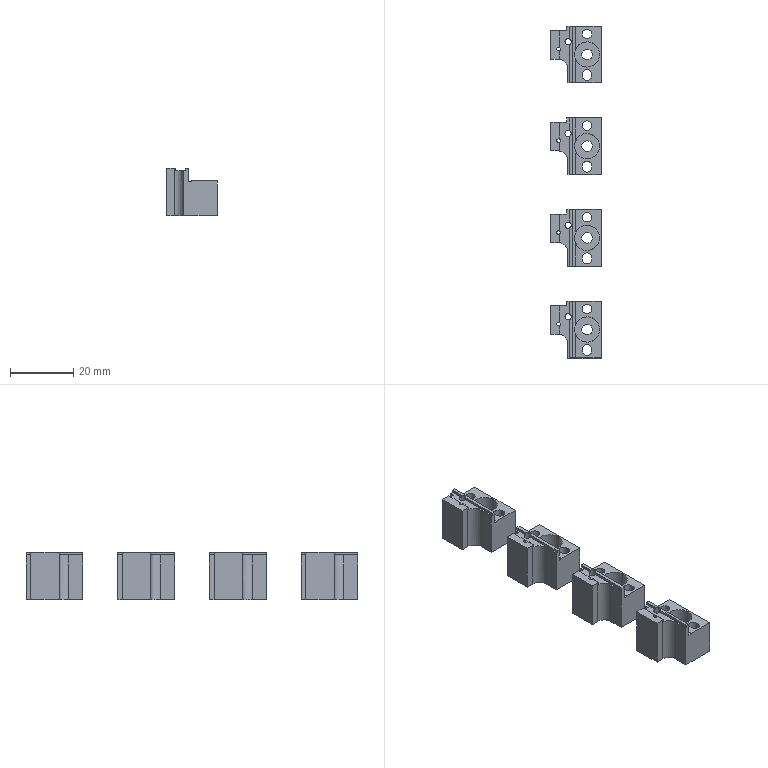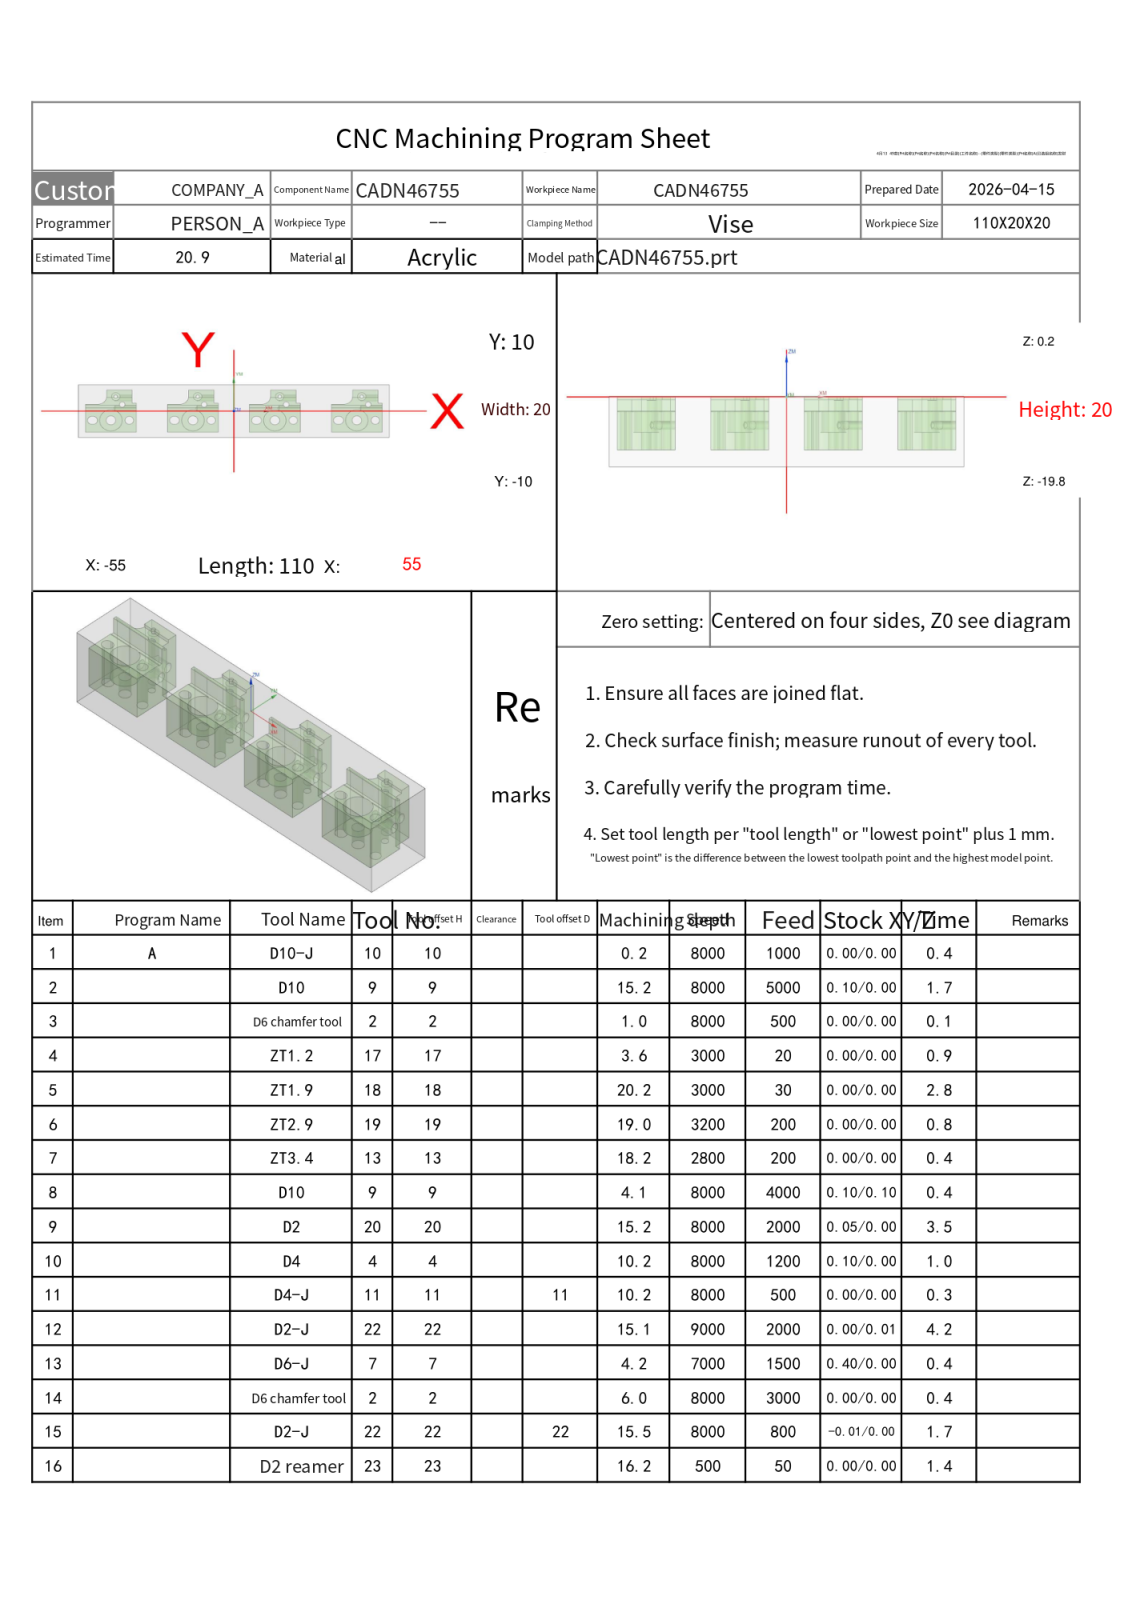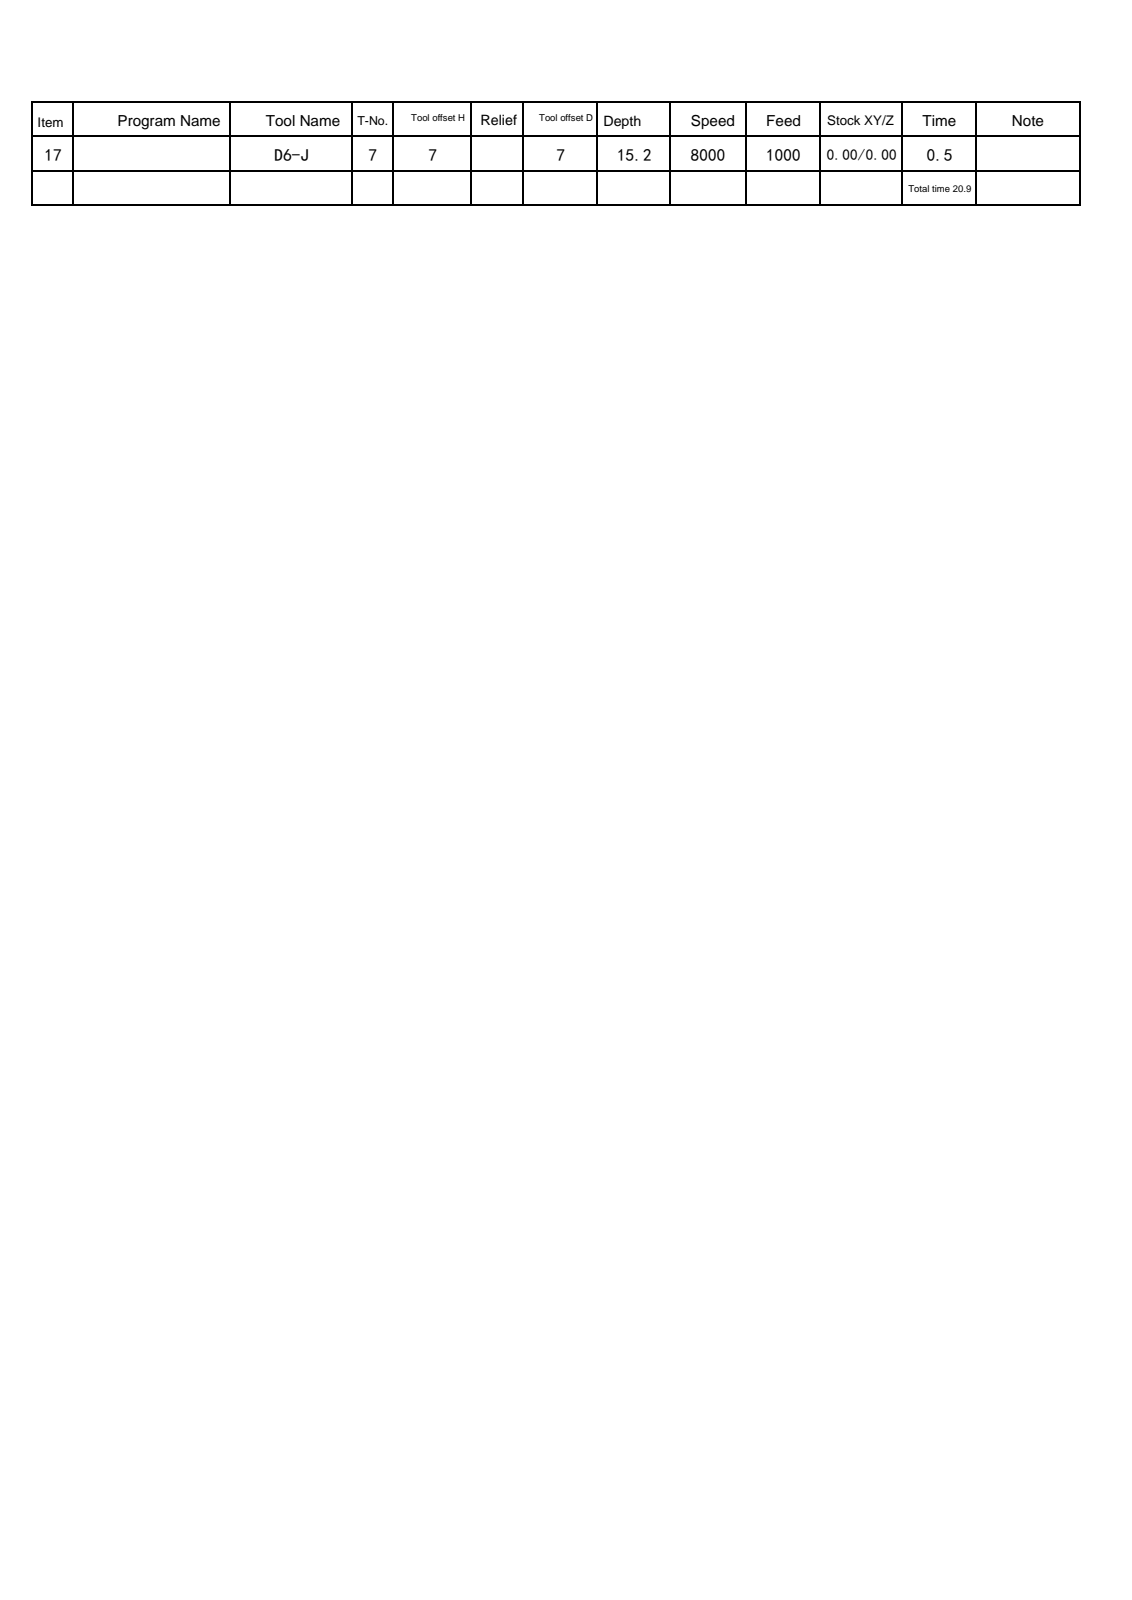NC program | NX | posted by the shop | part box 16 x 105 x 15 mm
Lines 5479 to 6592 of 25120:
N12 T22 M06
(D2-J  D=2. R=0. H=22 ce=0.00 di=0.01)
G00 G90 G54 X-46.858 Y4.697 M03 S9000
G43 H22 Z20.
M08
Z.601
G01 X-46.848 Z.486 F1600.
X-46.82 Y4.7 Z.384
X-46.778 Y4.706 Z.292
X-46.722 Y4.716 Z.211
X-46.657 Y4.731 Z.139
X-46.584 Y4.752 Z.077
X-46.506 Y4.779 Z.024
X-46.426 Y4.814 Z-.021
X-46.347 Y4.857 Z-.058
X-46.27 Y4.909 Z-.088
X-46.198 Y4.971 Z-.112
X-46.134 Y5.045 Z-.129
X-46.081 Y5.13 Z-.141
X-46.041 Y5.228 Z-.147
X-46.017 Y5.34 Z-.15
G03 X-46. Y5.6 I-1.983 J.26 F2000.
G01 Y7.3
X-46.007 Y7.322
X-46.026 Y7.315 Z-.153
X-46.054 Y7.283 Z-.157
X-46.089 Y7.228 Z-.162
X-46.128 Y7.154 Z-.168
X-46.167 Y7.064 Z-.174
X-46.205 Y6.96 Z-.182
X-46.239 Y6.847 Z-.19
X-46.286 Y6.601 Z-.207
X-46.304 Y6.34 Z-.224
X-46.293 Y6.077 Z-.242
X-46.254 Y5.825 Z-.259
X-46.223 Y5.707 Z-.267
X-46.188 Y5.599 Z-.274
X-46.15 Y5.503 Z-.281
X-46.113 Y5.424 Z-.287
X-46.078 Y5.365 Z-.292
X-46.049 Y5.329 Z-.296
X-46.028 Y5.319 Z-.298
X-46.017 Y5.34 Z-.299
G03 X-46. Y5.6 I-1.983 J.26
G01 Y7.3
X-46.007 Y7.322 Z-.3
X-46.026 Y7.315 Z-.302
X-46.054 Y7.283 Z-.306
X-46.089 Y7.228 Z-.311
X-46.128 Y7.154 Z-.317
X-46.167 Y7.064 Z-.324
X-46.205 Y6.96 Z-.331
X-46.239 Y6.847 Z-.339
X-46.286 Y6.601 Z-.356
X-46.304 Y6.34 Z-.374
X-46.293 Y6.077 Z-.391
X-46.254 Y5.825 Z-.408
X-46.223 Y5.707 Z-.416
X-46.188 Y5.599 Z-.424
X-46.15 Y5.503 Z-.43
X-46.113 Y5.424 Z-.436
X-46.078 Y5.365 Z-.441
X-46.049 Y5.329 Z-.445
X-46.028 Y5.319 Z-.448
X-46.017 Y5.34 Z-.449
G03 X-46. Y5.6 I-1.983 J.26
G01 Y7.3
X-46.007 Y7.322
X-46.026 Y7.315 Z-.452
X-46.054 Y7.283 Z-.456
X-46.089 Y7.228 Z-.461
X-46.128 Y7.154 Z-.467
X-46.167 Y7.064 Z-.473
X-46.205 Y6.96 Z-.481
X-46.239 Y6.847 Z-.489
X-46.286 Y6.601 Z-.506
X-46.304 Y6.34 Z-.523
X-46.293 Y6.077 Z-.541
X-46.254 Y5.825 Z-.558
X-46.223 Y5.707 Z-.566
X-46.188 Y5.599 Z-.573
X-46.15 Y5.503 Z-.58
X-46.113 Y5.424 Z-.586
X-46.078 Y5.365 Z-.591
X-46.049 Y5.329 Z-.595
X-46.028 Y5.319 Z-.597
X-46.017 Y5.34 Z-.598
G03 X-46. Y5.6 I-1.983 J.26
G01 Y7.3
X-46.007 Y7.322 Z-.599
X-46.026 Y7.315 Z-.601
X-46.054 Y7.283 Z-.605
X-46.089 Y7.228 Z-.61
X-46.128 Y7.154 Z-.616
X-46.167 Y7.064 Z-.623
X-46.205 Y6.96 Z-.63
X-46.239 Y6.847 Z-.638
X-46.286 Y6.601 Z-.655
X-46.304 Y6.34 Z-.673
X-46.293 Y6.077 Z-.69
X-46.254 Y5.825 Z-.707
X-46.223 Y5.707 Z-.715
X-46.188 Y5.599 Z-.723
X-46.15 Y5.503 Z-.729
X-46.113 Y5.424 Z-.735
X-46.078 Y5.365 Z-.74
X-46.049 Y5.329 Z-.744
X-46.028 Y5.319 Z-.747
X-46.017 Y5.34 Z-.748
G03 X-46. Y5.6 I-1.983 J.26
G01 Y7.3
X-46.016 Y7.315
X-46.061 Y7.307 Z-.749
X-46.132 Y7.278 Z-.751
X-46.228 Y7.23 Z-.754
X-46.483 Y7.077 Z-.762
X-46.829 Y6.848 Z-.773
X-47.215 Y6.572 Z-.785
X-47.805 Y6.108 Z-.805
X-48.29 Y5.688 Z-.822
X-48.757 Y5.248 Z-.84
X-49.231 Y4.758 Z-.858
X-49.573 Y4.37 Z-.872
X-49.839 Y4.044 Z-.883
X-50.012 Y3.809 Z-.89
X-50.068 Y3.722 Z-.893
X-50.102 Y3.656 Z-.895
X-50.113 Y3.614 Z-.897
X-50.1 Y3.6
X-48.
G03 X-46. Y5.6 I0.0 J2.
G01 Y7.7
X-46.016 Y7.713
X-46.061 Y7.702 Z-.899
X-46.132 Y7.668 Z-.901
X-46.227 Y7.612 Z-.904
X-46.545 Y7.393 Z-.913
X-46.84 Y7.17 Z-.922
X-47.213 Y6.871 Z-.934
X-47.803 Y6.354 Z-.954
X-48.289 Y5.887 Z-.972
X-48.755 Y5.402 Z-.989
X-49.272 Y4.812 Z-1.009
X-49.571 Y4.439 Z-1.021
X-49.794 Y4.144 Z-1.03
X-50.012 Y3.827 Z-1.04
X-50.068 Y3.732 Z-1.043
X-50.102 Y3.661 Z-1.045
X-50.113 Y3.616 Z-1.046
X-50.1 Y3.6 Z-1.047
X-48.
G03 X-46. Y5.6 I0.0 J2.
G01 Y7.7
X-46.016 Y7.713
X-46.061 Y7.702 Z-1.048
X-46.132 Y7.668 Z-1.05
X-46.227 Y7.612 Z-1.053
X-46.545 Y7.393 Z-1.063
X-46.84 Y7.17 Z-1.072
X-47.213 Y6.871 Z-1.084
X-47.803 Y6.354 Z-1.104
X-48.289 Y5.887 Z-1.121
X-48.755 Y5.402 Z-1.139
X-49.272 Y4.812 Z-1.159
X-49.571 Y4.439 Z-1.171
X-49.794 Y4.144 Z-1.18
X-50.012 Y3.827 Z-1.189
X-50.068 Y3.732 Z-1.192
X-50.102 Y3.661 Z-1.194
X-50.113 Y3.616 Z-1.196
X-50.1 Y3.6
X-48.
G03 X-46. Y5.6 I0.0 J2.
G01 Y7.7
X-46.016 Y7.713
X-46.061 Y7.702 Z-1.198
X-46.132 Y7.668 Z-1.2
X-46.227 Y7.612 Z-1.203
X-46.545 Y7.393 Z-1.212
X-46.84 Y7.17 Z-1.221
X-47.213 Y6.871 Z-1.233
X-47.803 Y6.354 Z-1.253
X-48.289 Y5.887 Z-1.271
X-48.755 Y5.402 Z-1.288
X-49.272 Y4.812 Z-1.308
X-49.571 Y4.439 Z-1.32
X-49.794 Y4.144 Z-1.329
X-50.012 Y3.827 Z-1.339
X-50.068 Y3.732 Z-1.342
X-50.102 Y3.661 Z-1.344
X-50.113 Y3.616 Z-1.345
X-50.1 Y3.6 Z-1.346
X-48.
G03 X-46. Y5.6 I0.0 J2.
G01 Y7.7
X-46.016 Y7.713
X-46.061 Y7.702 Z-1.347
X-46.132 Y7.668 Z-1.349
X-46.227 Y7.612 Z-1.352
X-46.545 Y7.393 Z-1.362
X-46.84 Y7.17 Z-1.371
X-47.213 Y6.871 Z-1.383
X-47.803 Y6.354 Z-1.403
X-48.289 Y5.887 Z-1.42
X-48.755 Y5.402 Z-1.438
X-49.272 Y4.812 Z-1.458
X-49.571 Y4.439 Z-1.47
X-49.794 Y4.144 Z-1.479
X-50.012 Y3.827 Z-1.488
X-50.068 Y3.732 Z-1.491
X-50.102 Y3.661 Z-1.493
X-50.113 Y3.616 Z-1.495
X-50.1 Y3.6
X-48.
G03 X-46. Y5.6 I0.0 J2.
G01 Y7.7
X-46.016 Y7.713
X-46.061 Y7.702 Z-1.497
X-46.132 Y7.668 Z-1.499
X-46.227 Y7.612 Z-1.502
X-46.545 Y7.393 Z-1.511
X-46.84 Y7.17 Z-1.52
X-47.213 Y6.871 Z-1.532
X-47.803 Y6.354 Z-1.552
X-48.289 Y5.887 Z-1.57
X-48.755 Y5.402 Z-1.587
X-49.272 Y4.812 Z-1.607
X-49.571 Y4.439 Z-1.619
X-49.794 Y4.144 Z-1.628
X-50.012 Y3.827 Z-1.638
X-50.068 Y3.732 Z-1.641
X-50.102 Y3.661 Z-1.643
X-50.113 Y3.616 Z-1.644
X-50.1 Y3.6 Z-1.645
X-48.
G03 X-46. Y5.6 I0.0 J2.
G01 Y7.7
X-46.016 Y7.713
X-46.061 Y7.702 Z-1.646
X-46.132 Y7.668 Z-1.648
X-46.227 Y7.612 Z-1.651
X-46.545 Y7.393 Z-1.661
X-46.84 Y7.17 Z-1.67
X-47.213 Y6.871 Z-1.682
X-47.803 Y6.354 Z-1.702
X-48.289 Y5.887 Z-1.719
X-48.755 Y5.402 Z-1.737
X-49.272 Y4.812 Z-1.757
X-49.571 Y4.439 Z-1.769
X-49.794 Y4.144 Z-1.778
X-50.012 Y3.827 Z-1.787
X-50.068 Y3.732 Z-1.79
X-50.102 Y3.661 Z-1.792
X-50.113 Y3.616 Z-1.794
X-50.1 Y3.6
X-48.
G03 X-46. Y5.6 I0.0 J2.
G01 Y7.7
X-46.016 Y7.713
X-46.061 Y7.702 Z-1.796
X-46.132 Y7.668 Z-1.798
X-46.227 Y7.612 Z-1.801
X-46.545 Y7.393 Z-1.81
X-46.84 Y7.17 Z-1.819
X-47.213 Y6.871 Z-1.831
X-47.803 Y6.354 Z-1.851
X-48.289 Y5.887 Z-1.869
X-48.755 Y5.402 Z-1.886
X-49.272 Y4.812 Z-1.906
X-49.571 Y4.439 Z-1.918
X-49.794 Y4.144 Z-1.927
X-50.012 Y3.827 Z-1.937
X-50.068 Y3.732 Z-1.94
X-50.102 Y3.661 Z-1.942
X-50.113 Y3.616 Z-1.943
X-50.1 Y3.6 Z-1.944
X-48.
G03 X-46. Y5.6 I0.0 J2.
G01 Y7.7
X-46.016 Y7.713
X-46.061 Y7.702 Z-1.945
X-46.132 Y7.668 Z-1.947
X-46.227 Y7.612 Z-1.95
X-46.545 Y7.393 Z-1.96
X-46.84 Y7.17 Z-1.969
X-47.213 Y6.871 Z-1.981
X-47.803 Y6.354 Z-2.001
X-48.289 Y5.887 Z-2.018
X-48.755 Y5.402 Z-2.036
X-49.272 Y4.812 Z-2.056
X-49.571 Y4.439 Z-2.068
X-49.794 Y4.144 Z-2.077
X-50.012 Y3.827 Z-2.086
X-50.068 Y3.732 Z-2.089
X-50.102 Y3.661 Z-2.091
X-50.113 Y3.616 Z-2.093
X-50.1 Y3.6
X-48.
G03 X-46. Y5.6 I0.0 J2.
G01 Y7.7
X-46.016 Y7.713
X-46.061 Y7.702 Z-2.095
X-46.132 Y7.668 Z-2.097
X-46.227 Y7.612 Z-2.1
X-46.545 Y7.393 Z-2.109
X-46.84 Y7.17 Z-2.118
X-47.213 Y6.871 Z-2.13
X-47.803 Y6.354 Z-2.15
X-48.289 Y5.887 Z-2.168
X-48.755 Y5.402 Z-2.185
X-49.272 Y4.812 Z-2.205
X-49.571 Y4.439 Z-2.217
X-49.794 Y4.144 Z-2.226
X-50.012 Y3.827 Z-2.236
X-50.068 Y3.732 Z-2.239
X-50.102 Y3.661 Z-2.241
X-50.113 Y3.616 Z-2.242
X-50.1 Y3.6 Z-2.243
X-48.
G03 X-46. Y5.6 I0.0 J2.
G01 Y7.7
X-46.016 Y7.713
X-46.061 Y7.702 Z-2.244
X-46.132 Y7.668 Z-2.246
X-46.227 Y7.612 Z-2.249
X-46.545 Y7.393 Z-2.259
X-46.84 Y7.17 Z-2.268
X-47.213 Y6.871 Z-2.28
X-47.803 Y6.354 Z-2.3
X-48.289 Y5.887 Z-2.317
X-48.755 Y5.402 Z-2.335
X-49.272 Y4.812 Z-2.355
X-49.571 Y4.439 Z-2.367
X-49.794 Y4.144 Z-2.376
X-50.012 Y3.827 Z-2.385
X-50.068 Y3.732 Z-2.388
X-50.102 Y3.661 Z-2.39
X-50.113 Y3.616 Z-2.392
X-50.1 Y3.6
X-48.
G03 X-46. Y5.6 I0.0 J2.
G01 Y7.7
X-46.016 Y7.713
X-46.061 Y7.702 Z-2.394
X-46.132 Y7.668 Z-2.396
X-46.227 Y7.612 Z-2.399
X-46.545 Y7.393 Z-2.408
X-46.84 Y7.17 Z-2.417
X-47.213 Y6.871 Z-2.429
X-47.803 Y6.354 Z-2.449
X-48.289 Y5.887 Z-2.467
X-48.755 Y5.402 Z-2.484
X-49.272 Y4.812 Z-2.504
X-49.571 Y4.439 Z-2.516
X-49.794 Y4.144 Z-2.525
X-50.012 Y3.827 Z-2.535
X-50.068 Y3.732 Z-2.538
X-50.102 Y3.661 Z-2.54
X-50.113 Y3.616 Z-2.541
X-50.1 Y3.6 Z-2.542
X-48.
G03 X-46. Y5.6 I0.0 J2.
G01 Y7.7
X-46.016 Y7.713
X-46.061 Y7.702 Z-2.543
X-46.132 Y7.668 Z-2.545
X-46.227 Y7.612 Z-2.548
X-46.545 Y7.393 Z-2.558
X-46.84 Y7.17 Z-2.567
X-47.213 Y6.871 Z-2.579
X-47.803 Y6.354 Z-2.599
X-48.289 Y5.887 Z-2.616
X-48.755 Y5.402 Z-2.634
X-49.272 Y4.812 Z-2.654
X-49.571 Y4.439 Z-2.666
X-49.794 Y4.144 Z-2.675
X-50.012 Y3.827 Z-2.684
X-50.068 Y3.732 Z-2.687
X-50.102 Y3.661 Z-2.689
X-50.113 Y3.616 Z-2.691
X-50.1 Y3.6
X-48.
G03 X-46. Y5.6 I0.0 J2.
G01 Y7.7
X-46.016 Y7.713
X-46.061 Y7.702 Z-2.693
X-46.132 Y7.668 Z-2.695
X-46.227 Y7.612 Z-2.698
X-46.545 Y7.393 Z-2.707
X-46.84 Y7.17 Z-2.716
X-47.213 Y6.871 Z-2.728
X-47.803 Y6.354 Z-2.748
X-48.289 Y5.887 Z-2.766
X-48.755 Y5.402 Z-2.783
X-49.272 Y4.812 Z-2.803
X-49.571 Y4.439 Z-2.815
X-49.794 Y4.144 Z-2.824
X-50.012 Y3.827 Z-2.834
X-50.068 Y3.732 Z-2.837
X-50.102 Y3.661 Z-2.839
X-50.113 Y3.616 Z-2.84
X-50.1 Y3.6 Z-2.841
X-48.
G03 X-46. Y5.6 I0.0 J2.
G01 Y7.7
X-46.016 Y7.713
X-46.061 Y7.702 Z-2.842
X-46.132 Y7.668 Z-2.844
X-46.227 Y7.612 Z-2.847
X-46.545 Y7.393 Z-2.857
X-46.84 Y7.17 Z-2.866
X-47.213 Y6.871 Z-2.878
X-47.803 Y6.354 Z-2.898
X-48.289 Y5.887 Z-2.915
X-48.755 Y5.402 Z-2.933
X-49.272 Y4.812 Z-2.953
X-49.571 Y4.439 Z-2.965
X-49.794 Y4.144 Z-2.974
X-50.012 Y3.827 Z-2.983
X-50.068 Y3.732 Z-2.986
X-50.102 Y3.661 Z-2.988
X-50.113 Y3.616 Z-2.99
X-50.1 Y3.6
X-48.
G03 X-46. Y5.6 I0.0 J2.
G01 Y7.7
X-46.016 Y7.713
X-46.061 Y7.702 Z-2.992
X-46.132 Y7.668 Z-2.994
X-46.227 Y7.612 Z-2.997
X-46.545 Y7.393 Z-3.006
X-46.84 Y7.17 Z-3.015
X-47.213 Y6.871 Z-3.027
X-47.803 Y6.354 Z-3.047
X-48.289 Y5.887 Z-3.065
X-48.755 Y5.402 Z-3.082
X-49.272 Y4.812 Z-3.102
X-49.571 Y4.439 Z-3.114
X-49.794 Y4.144 Z-3.123
X-50.012 Y3.827 Z-3.133
X-50.068 Y3.732 Z-3.136
X-50.102 Y3.661 Z-3.138
X-50.113 Y3.616 Z-3.139
X-50.1 Y3.6 Z-3.14
X-48.
G03 X-46. Y5.6 I0.0 J2.
G01 Y7.7
X-46.016 Y7.713
X-46.061 Y7.702 Z-3.141
X-46.132 Y7.668 Z-3.143
X-46.227 Y7.612 Z-3.146
X-46.545 Y7.393 Z-3.156
X-46.84 Y7.17 Z-3.165
X-47.213 Y6.871 Z-3.177
X-47.803 Y6.354 Z-3.197
X-48.289 Y5.887 Z-3.214
X-48.755 Y5.402 Z-3.232
X-49.272 Y4.812 Z-3.252
X-49.571 Y4.439 Z-3.264
X-49.794 Y4.144 Z-3.273
X-50.012 Y3.827 Z-3.282
X-50.068 Y3.732 Z-3.285
X-50.102 Y3.661 Z-3.287
X-50.113 Y3.616 Z-3.289
X-50.1 Y3.6
X-48.
G03 X-46. Y5.6 I0.0 J2.
G01 Y7.7
X-46.016 Y7.713
X-46.061 Y7.702 Z-3.291
X-46.132 Y7.668 Z-3.293
X-46.227 Y7.612 Z-3.296
X-46.545 Y7.393 Z-3.305
X-46.84 Y7.17 Z-3.314
X-47.213 Y6.871 Z-3.326
X-47.803 Y6.354 Z-3.346
X-48.289 Y5.887 Z-3.364
X-48.755 Y5.402 Z-3.381
X-49.272 Y4.812 Z-3.401
X-49.571 Y4.439 Z-3.413
X-49.794 Y4.144 Z-3.422
X-50.012 Y3.827 Z-3.432
X-50.068 Y3.732 Z-3.435
X-50.102 Y3.661 Z-3.437
X-50.113 Y3.616 Z-3.438
X-50.1 Y3.6 Z-3.439
X-48.
G03 X-46. Y5.6 I0.0 J2.
G01 Y7.7
X-46.016 Y7.713
X-46.061 Y7.702 Z-3.44
X-46.132 Y7.668 Z-3.442
X-46.227 Y7.612 Z-3.445
X-46.545 Y7.393 Z-3.455
X-46.84 Y7.17 Z-3.464
X-47.213 Y6.871 Z-3.476
X-47.803 Y6.354 Z-3.496
X-48.289 Y5.887 Z-3.513
X-48.755 Y5.402 Z-3.531
X-49.272 Y4.812 Z-3.551
X-49.571 Y4.439 Z-3.563
X-49.794 Y4.144 Z-3.572
X-50.012 Y3.827 Z-3.581
X-50.068 Y3.732 Z-3.584
X-50.102 Y3.661 Z-3.586
X-50.113 Y3.616 Z-3.588
X-50.1 Y3.6
X-48.
G03 X-46. Y5.6 I0.0 J2.
G01 Y7.7
X-46.016 Y7.713
X-46.061 Y7.702 Z-3.59
X-46.132 Y7.668 Z-3.592
X-46.227 Y7.612 Z-3.595
X-46.545 Y7.393 Z-3.604
X-46.84 Y7.17 Z-3.613
X-47.213 Y6.871 Z-3.625
X-47.803 Y6.354 Z-3.645
X-48.289 Y5.887 Z-3.663
X-48.755 Y5.402 Z-3.68
X-49.272 Y4.812 Z-3.7
X-49.571 Y4.439 Z-3.712
X-49.794 Y4.144 Z-3.721
X-50.012 Y3.827 Z-3.731
X-50.068 Y3.732 Z-3.734
X-50.102 Y3.661 Z-3.736
X-50.113 Y3.616 Z-3.737
X-50.1 Y3.6 Z-3.738
X-48.
G03 X-46. Y5.6 I0.0 J2.
G01 Y7.7
X-46.016 Y7.713
X-46.061 Y7.702 Z-3.739
X-46.132 Y7.668 Z-3.741
X-46.227 Y7.612 Z-3.744
X-46.545 Y7.393 Z-3.754
X-46.84 Y7.17 Z-3.763
X-47.213 Y6.871 Z-3.775
X-47.803 Y6.354 Z-3.795
X-48.289 Y5.887 Z-3.812
X-48.755 Y5.402 Z-3.83
X-49.272 Y4.812 Z-3.85
X-49.571 Y4.439 Z-3.862
X-49.794 Y4.144 Z-3.871
X-50.012 Y3.827 Z-3.88
X-50.068 Y3.732 Z-3.883
X-50.102 Y3.661 Z-3.885
X-50.113 Y3.616 Z-3.887
X-50.1 Y3.6
X-48.
G03 X-46. Y5.6 I0.0 J2.
G01 Y7.7
X-46.016 Y7.713
X-46.061 Y7.702 Z-3.889
X-46.132 Y7.668 Z-3.891
X-46.227 Y7.612 Z-3.894
X-46.545 Y7.393 Z-3.903
X-46.84 Y7.17 Z-3.912
X-47.213 Y6.871 Z-3.924
X-47.803 Y6.354 Z-3.944
X-48.289 Y5.887 Z-3.962
X-48.755 Y5.402 Z-3.979
X-49.272 Y4.812 Z-3.999
X-49.571 Y4.439 Z-4.011
X-49.794 Y4.144 Z-4.02
X-50.012 Y3.827 Z-4.03
X-50.068 Y3.732 Z-4.033
X-50.102 Y3.661 Z-4.035
X-50.113 Y3.616 Z-4.036
X-50.1 Y3.6 Z-4.037
X-48.
G03 X-46. Y5.6 I0.0 J2.
G01 Y7.7
X-46.016 Y7.713
X-46.061 Y7.702 Z-4.038
X-46.132 Y7.668 Z-4.04
X-46.227 Y7.612 Z-4.043
X-46.545 Y7.393 Z-4.053
X-46.84 Y7.17 Z-4.062
X-47.213 Y6.871 Z-4.074
X-47.803 Y6.354 Z-4.094
X-48.289 Y5.887 Z-4.111
X-48.755 Y5.402 Z-4.129
X-49.272 Y4.812 Z-4.149
X-49.571 Y4.439 Z-4.161
X-49.794 Y4.144 Z-4.17
X-50.012 Y3.827 Z-4.179
X-50.068 Y3.732 Z-4.182
X-50.102 Y3.661 Z-4.184
X-50.113 Y3.616 Z-4.186
X-50.1 Y3.6
X-48.
G03 X-46. Y5.6 I0.0 J2.
G01 Y7.7
X-46.016 Y7.713
X-46.061 Y7.702 Z-4.188
X-46.132 Y7.668 Z-4.19
X-46.227 Y7.612 Z-4.193
X-46.545 Y7.393 Z-4.202
X-46.84 Y7.17 Z-4.211
X-47.213 Y6.871 Z-4.223
X-47.803 Y6.354 Z-4.243
X-48.289 Y5.887 Z-4.261
X-48.755 Y5.402 Z-4.278
X-49.272 Y4.812 Z-4.298
X-49.571 Y4.439 Z-4.31
X-49.794 Y4.144 Z-4.319
X-50.012 Y3.827 Z-4.329
X-50.068 Y3.732 Z-4.332
X-50.102 Y3.661 Z-4.334
X-50.113 Y3.616 Z-4.335
X-50.1 Y3.6 Z-4.336
X-48.
G03 X-46. Y5.6 I0.0 J2.
G01 Y7.7
X-46.016 Y7.713
X-46.061 Y7.702 Z-4.337
X-46.132 Y7.668 Z-4.339
X-46.227 Y7.612 Z-4.342
X-46.545 Y7.393 Z-4.352
X-46.84 Y7.17 Z-4.361
X-47.213 Y6.871 Z-4.373
X-47.803 Y6.354 Z-4.393
X-48.289 Y5.887 Z-4.41
X-48.755 Y5.402 Z-4.428
X-49.272 Y4.812 Z-4.448
X-49.571 Y4.439 Z-4.46
X-49.794 Y4.144 Z-4.469
X-50.012 Y3.827 Z-4.478
X-50.068 Y3.732 Z-4.481
X-50.102 Y3.661 Z-4.483
X-50.113 Y3.616 Z-4.485
X-50.1 Y3.6
X-48.
G03 X-46. Y5.6 I0.0 J2.
G01 Y7.7
X-46.016 Y7.713
X-46.061 Y7.702 Z-4.487
X-46.132 Y7.668 Z-4.489
X-46.227 Y7.612 Z-4.492
X-46.545 Y7.393 Z-4.501
X-46.84 Y7.17 Z-4.51
X-47.213 Y6.871 Z-4.522
X-47.803 Y6.354 Z-4.542
X-48.289 Y5.887 Z-4.56
X-48.755 Y5.402 Z-4.577
X-49.272 Y4.812 Z-4.597
X-49.571 Y4.439 Z-4.609
X-49.794 Y4.144 Z-4.618
X-50.012 Y3.827 Z-4.628
X-50.068 Y3.732 Z-4.631
X-50.102 Y3.661 Z-4.633
X-50.113 Y3.616 Z-4.634
X-50.1 Y3.6 Z-4.635
X-48.
G03 X-46. Y5.6 I0.0 J2.
G01 Y7.7
X-46.016 Y7.713
X-46.061 Y7.702 Z-4.636
X-46.132 Y7.668 Z-4.638
X-46.227 Y7.612 Z-4.641
X-46.545 Y7.393 Z-4.651
X-46.84 Y7.17 Z-4.66
X-47.213 Y6.871 Z-4.672
X-47.803 Y6.354 Z-4.692
X-48.289 Y5.887 Z-4.709
X-48.755 Y5.402 Z-4.727
X-49.272 Y4.812 Z-4.747
X-49.571 Y4.439 Z-4.759
X-49.794 Y4.144 Z-4.768
X-50.012 Y3.827 Z-4.777
X-50.068 Y3.732 Z-4.78
X-50.102 Y3.661 Z-4.782
X-50.113 Y3.616 Z-4.784
X-50.1 Y3.6
X-48.
G03 X-46. Y5.6 I0.0 J2.
G01 Y7.7
X-46.016 Y7.713
X-46.061 Y7.702 Z-4.786
X-46.132 Y7.668 Z-4.788
X-46.227 Y7.612 Z-4.791
X-46.545 Y7.393 Z-4.8
X-46.84 Y7.17 Z-4.809
X-47.213 Y6.871 Z-4.821
X-47.803 Y6.354 Z-4.841
X-48.289 Y5.887 Z-4.859
X-48.755 Y5.402 Z-4.876
X-49.272 Y4.812 Z-4.896
X-49.571 Y4.439 Z-4.908
X-49.794 Y4.144 Z-4.917
X-50.012 Y3.827 Z-4.927
X-50.068 Y3.732 Z-4.93
X-50.102 Y3.661 Z-4.932
X-50.113 Y3.616 Z-4.933
X-50.1 Y3.6 Z-4.934
X-48.
G03 X-46. Y5.6 I0.0 J2.
G01 Y7.7
X-46.016 Y7.713
X-46.061 Y7.702 Z-4.935
X-46.132 Y7.668 Z-4.937
X-46.227 Y7.612 Z-4.94
X-46.545 Y7.393 Z-4.95
X-46.84 Y7.17 Z-4.959
X-47.213 Y6.871 Z-4.971
X-47.803 Y6.354 Z-4.991
X-48.289 Y5.887 Z-5.008
X-48.755 Y5.402 Z-5.026
X-49.272 Y4.812 Z-5.046
X-49.571 Y4.439 Z-5.058
X-49.794 Y4.144 Z-5.067
X-50.012 Y3.827 Z-5.076
X-50.068 Y3.732 Z-5.079
X-50.102 Y3.661 Z-5.081
X-50.113 Y3.616 Z-5.083
X-50.1 Y3.6
X-48.
G03 X-46. Y5.6 I0.0 J2.
G01 Y7.7
X-46.016 Y7.713
X-46.061 Y7.702 Z-5.085
X-46.132 Y7.668 Z-5.087
X-46.227 Y7.612 Z-5.09
X-46.545 Y7.393 Z-5.099
X-46.84 Y7.17 Z-5.108
X-47.213 Y6.871 Z-5.12
X-47.803 Y6.354 Z-5.14
X-48.289 Y5.887 Z-5.158
X-48.755 Y5.402 Z-5.175
X-49.272 Y4.812 Z-5.195
X-49.571 Y4.439 Z-5.207
X-49.794 Y4.144 Z-5.216
X-50.012 Y3.827 Z-5.226
X-50.068 Y3.732 Z-5.229
X-50.102 Y3.661 Z-5.231
X-50.113 Y3.616 Z-5.232
X-50.1 Y3.6 Z-5.233
X-48.
G03 X-46. Y5.6 I0.0 J2.
G01 Y7.7
X-46.016 Y7.713
X-46.061 Y7.702 Z-5.234
X-46.132 Y7.668 Z-5.236
X-46.227 Y7.612 Z-5.239
X-46.545 Y7.393 Z-5.249
X-46.84 Y7.17 Z-5.258
X-47.213 Y6.871 Z-5.27
X-47.803 Y6.354 Z-5.29
X-48.289 Y5.887 Z-5.307
X-48.755 Y5.402 Z-5.325
X-49.272 Y4.812 Z-5.345
X-49.571 Y4.439 Z-5.357
X-49.794 Y4.144 Z-5.366
X-50.012 Y3.827 Z-5.375
X-50.068 Y3.732 Z-5.378
X-50.102 Y3.661 Z-5.38
X-50.113 Y3.616 Z-5.382
X-50.1 Y3.6
X-48.
G03 X-46. Y5.6 I0.0 J2.
G01 Y7.7
X-46.016 Y7.713
X-46.061 Y7.702 Z-5.384
X-46.132 Y7.668 Z-5.386
X-46.227 Y7.612 Z-5.389
X-46.545 Y7.393 Z-5.398
X-46.84 Y7.17 Z-5.407
X-47.213 Y6.871 Z-5.419
X-47.803 Y6.354 Z-5.439
X-48.289 Y5.887 Z-5.457
X-48.755 Y5.402 Z-5.474
X-49.272 Y4.812 Z-5.494
X-49.571 Y4.439 Z-5.506
X-49.794 Y4.144 Z-5.515
X-50.012 Y3.827 Z-5.525
X-50.068 Y3.732 Z-5.528
X-50.102 Y3.661 Z-5.53
X-50.113 Y3.616 Z-5.531
X-50.1 Y3.6 Z-5.532
X-48.
G03 X-46. Y5.6 I0.0 J2.
G01 Y7.7
X-46.016 Y7.713
X-46.061 Y7.702 Z-5.533
X-46.132 Y7.668 Z-5.535
X-46.227 Y7.612 Z-5.538
X-46.545 Y7.393 Z-5.548
X-46.84 Y7.17 Z-5.557
X-47.213 Y6.871 Z-5.569
X-47.803 Y6.354 Z-5.589
X-48.289 Y5.887 Z-5.606
X-48.755 Y5.402 Z-5.624
X-49.272 Y4.812 Z-5.644
X-49.571 Y4.439 Z-5.656
X-49.794 Y4.144 Z-5.665
X-50.012 Y3.827 Z-5.674
X-50.068 Y3.732 Z-5.677
X-50.102 Y3.661 Z-5.679
X-50.113 Y3.616 Z-5.681
X-50.1 Y3.6
X-48.
G03 X-46. Y5.6 I0.0 J2.
G01 Y7.7
X-46.016 Y7.713
X-46.061 Y7.702 Z-5.683
X-46.132 Y7.668 Z-5.685
X-46.227 Y7.612 Z-5.688
X-46.545 Y7.393 Z-5.697
X-46.84 Y7.17 Z-5.706
X-47.213 Y6.871 Z-5.718
X-47.803 Y6.354 Z-5.738
X-48.289 Y5.887 Z-5.756
X-48.755 Y5.402 Z-5.773
X-49.272 Y4.812 Z-5.793
X-49.571 Y4.439 Z-5.805
X-49.794 Y4.144 Z-5.814
X-50.012 Y3.827 Z-5.824
X-50.068 Y3.732 Z-5.827
X-50.102 Y3.661 Z-5.829
X-50.113 Y3.616 Z-5.83
X-50.1 Y3.6 Z-5.831
X-48.
G03 X-46. Y5.6 I0.0 J2.
G01 Y7.7
X-46.016 Y7.713
X-46.061 Y7.702 Z-5.832
X-46.132 Y7.668 Z-5.834
X-46.227 Y7.612 Z-5.837
X-46.545 Y7.393 Z-5.847
X-46.84 Y7.17 Z-5.856
X-47.213 Y6.871 Z-5.868
X-47.803 Y6.354 Z-5.888
X-48.289 Y5.887 Z-5.905
X-48.755 Y5.402 Z-5.923
X-49.272 Y4.812 Z-5.943
X-49.571 Y4.439 Z-5.955
X-49.794 Y4.144 Z-5.964
X-50.012 Y3.827 Z-5.973
X-50.068 Y3.732 Z-5.976
X-50.102 Y3.661 Z-5.978
X-50.113 Y3.616 Z-5.98
X-50.1 Y3.6
X-48.
G03 X-46. Y5.6 I0.0 J2.
G01 Y7.7
X-46.016 Y7.713
X-46.061 Y7.702 Z-5.982
X-46.132 Y7.668 Z-5.984
X-46.227 Y7.612 Z-5.987
X-46.545 Y7.393 Z-5.996
X-46.84 Y7.17 Z-6.005
X-47.213 Y6.871 Z-6.017
X-47.803 Y6.354 Z-6.037
X-48.289 Y5.887 Z-6.055
X-48.755 Y5.402 Z-6.072
X-49.272 Y4.812 Z-6.092
X-49.571 Y4.439 Z-6.104
X-49.794 Y4.144 Z-6.113
X-50.012 Y3.827 Z-6.123
X-50.068 Y3.732 Z-6.126
X-50.102 Y3.661 Z-6.128
X-50.113 Y3.616 Z-6.129
X-50.1 Y3.6 Z-6.13
X-48.
G03 X-46. Y5.6 I0.0 J2.
G01 Y7.7
X-46.016 Y7.713
X-46.061 Y7.702 Z-6.131
X-46.132 Y7.668 Z-6.133
X-46.227 Y7.612 Z-6.136
X-46.545 Y7.393 Z-6.146
X-46.84 Y7.17 Z-6.155
X-47.213 Y6.871 Z-6.167
X-47.803 Y6.354 Z-6.187
X-48.289 Y5.887 Z-6.204
X-48.755 Y5.402 Z-6.222
X-49.272 Y4.812 Z-6.242
X-49.571 Y4.439 Z-6.254
X-49.794 Y4.144 Z-6.263
X-50.012 Y3.827 Z-6.272
X-50.068 Y3.732 Z-6.275
X-50.102 Y3.661 Z-6.277
X-50.113 Y3.616 Z-6.279
X-50.1 Y3.6
X-48.
G03 X-46. Y5.6 I0.0 J2.
G01 Y7.7
X-46.016 Y7.713
X-46.061 Y7.702 Z-6.281
X-46.132 Y7.668 Z-6.283
X-46.227 Y7.612 Z-6.286
X-46.545 Y7.393 Z-6.295
X-46.84 Y7.17 Z-6.304
X-47.213 Y6.871 Z-6.316
X-47.803 Y6.354 Z-6.336
X-48.289 Y5.887 Z-6.354
X-48.755 Y5.402 Z-6.371
X-49.272 Y4.812 Z-6.391
X-49.571 Y4.439 Z-6.403
X-49.794 Y4.144 Z-6.412
X-50.012 Y3.827 Z-6.422
X-50.068 Y3.732 Z-6.425
X-50.102 Y3.661 Z-6.427
X-50.113 Y3.616 Z-6.428
X-50.1 Y3.6 Z-6.429
X-48.
G03 X-46. Y5.6 I0.0 J2.
G01 Y7.7
X-46.016 Y7.713
X-46.061 Y7.702 Z-6.43
X-46.132 Y7.668 Z-6.432
X-46.227 Y7.612 Z-6.435
X-46.545 Y7.393 Z-6.445
X-46.84 Y7.17 Z-6.454
X-47.213 Y6.871 Z-6.466
X-47.803 Y6.354 Z-6.486
X-48.289 Y5.887 Z-6.503
X-48.755 Y5.402 Z-6.521
X-49.272 Y4.812 Z-6.541
X-49.571 Y4.439 Z-6.553
X-49.794 Y4.144 Z-6.562
X-50.012 Y3.827 Z-6.571
X-50.068 Y3.732 Z-6.574
X-50.102 Y3.661 Z-6.576
X-50.113 Y3.616 Z-6.578
X-50.1 Y3.6
X-48.
G03 X-46. Y5.6 I0.0 J2.
G01 Y7.7
X-46.016 Y7.713
X-46.061 Y7.702 Z-6.58
X-46.132 Y7.668 Z-6.582
X-46.227 Y7.612 Z-6.585
X-46.545 Y7.393 Z-6.594
X-46.84 Y7.17 Z-6.603
X-47.213 Y6.871 Z-6.615
X-47.803 Y6.354 Z-6.635
X-48.289 Y5.887 Z-6.653
X-48.755 Y5.402 Z-6.67
X-49.272 Y4.812 Z-6.69
X-49.571 Y4.439 Z-6.702
X-49.794 Y4.144 Z-6.711
X-50.012 Y3.827 Z-6.721
X-50.068 Y3.732 Z-6.724
X-50.102 Y3.661 Z-6.726
X-50.113 Y3.616 Z-6.727
X-50.1 Y3.6 Z-6.728
X-48.
G03 X-46. Y5.6 I0.0 J2.
G01 Y7.7
X-46.016 Y7.713
X-46.061 Y7.702 Z-6.729
X-46.132 Y7.668 Z-6.731
X-46.227 Y7.612 Z-6.734
X-46.545 Y7.393 Z-6.744
X-46.84 Y7.17 Z-6.753
X-47.213 Y6.871 Z-6.765
X-47.803 Y6.354 Z-6.785
X-48.289 Y5.887 Z-6.802
X-48.755 Y5.402 Z-6.82
X-49.272 Y4.812 Z-6.84
X-49.571 Y4.439 Z-6.852
X-49.794 Y4.144 Z-6.861
X-50.012 Y3.827 Z-6.87
X-50.068 Y3.732 Z-6.873
X-50.102 Y3.661 Z-6.875
X-50.113 Y3.616 Z-6.877
X-50.1 Y3.6
X-48.
G03 X-46. Y5.6 I0.0 J2.
G01 Y7.7
X-46.016 Y7.713
X-46.061 Y7.702 Z-6.879
X-46.132 Y7.668 Z-6.881
X-46.227 Y7.612 Z-6.884
X-46.545 Y7.393 Z-6.893
X-46.84 Y7.17 Z-6.902
X-47.213 Y6.871 Z-6.914
X-47.803 Y6.354 Z-6.934
X-48.289 Y5.887 Z-6.952
X-48.755 Y5.402 Z-6.969
X-49.272 Y4.812 Z-6.989
X-49.571 Y4.439 Z-7.001
X-49.794 Y4.144 Z-7.01
X-50.012 Y3.827 Z-7.02
X-50.068 Y3.732 Z-7.023
X-50.102 Y3.661 Z-7.025
X-50.113 Y3.616 Z-7.026
X-50.1 Y3.6 Z-7.027
X-48.
G03 X-46. Y5.6 I0.0 J2.
G01 Y7.7
X-46.016 Y7.713
X-46.061 Y7.702 Z-7.028
X-46.132 Y7.668 Z-7.03
X-46.227 Y7.612 Z-7.033
X-46.545 Y7.393 Z-7.043
X-46.84 Y7.17 Z-7.052
X-47.213 Y6.871 Z-7.064
X-47.803 Y6.354 Z-7.084
X-48.289 Y5.887 Z-7.101
X-48.755 Y5.402 Z-7.119
X-49.272 Y4.812 Z-7.139
X-49.571 Y4.439 Z-7.151
X-49.794 Y4.144 Z-7.16
X-50.012 Y3.827 Z-7.169
X-50.068 Y3.732 Z-7.172
X-50.102 Y3.661 Z-7.174
X-50.113 Y3.616 Z-7.176
X-50.1 Y3.6
X-48.
G03 X-46. Y5.6 I0.0 J2.
G01 Y7.7
X-46.016 Y7.713
X-46.061 Y7.702 Z-7.178
X-46.132 Y7.668 Z-7.18
X-46.227 Y7.612 Z-7.183
X-46.545 Y7.393 Z-7.192
X-46.84 Y7.17 Z-7.201
X-47.213 Y6.871 Z-7.213
X-47.803 Y6.354 Z-7.233
X-48.289 Y5.887 Z-7.251
X-48.755 Y5.402 Z-7.268
X-49.272 Y4.812 Z-7.288
X-49.571 Y4.439 Z-7.3
X-49.794 Y4.144 Z-7.309
X-50.012 Y3.827 Z-7.319
X-50.068 Y3.732 Z-7.322
X-50.102 Y3.661 Z-7.324
X-50.113 Y3.616 Z-7.325
X-50.1 Y3.6 Z-7.326
X-48.
G03 X-46. Y5.6 I0.0 J2.
G01 Y7.7
X-46.016 Y7.713
X-46.061 Y7.702 Z-7.327
X-46.132 Y7.668 Z-7.329
X-46.227 Y7.612 Z-7.332
X-46.545 Y7.393 Z-7.342
X-46.84 Y7.17 Z-7.351
X-47.213 Y6.871 Z-7.363
X-47.803 Y6.354 Z-7.383
X-48.289 Y5.887 Z-7.4
X-48.755 Y5.402 Z-7.418
X-49.272 Y4.812 Z-7.438
X-49.571 Y4.439 Z-7.45
X-49.794 Y4.144 Z-7.459
X-50.012 Y3.827 Z-7.468
X-50.068 Y3.732 Z-7.471
X-50.102 Y3.661 Z-7.473
X-50.113 Y3.616 Z-7.475
X-50.1 Y3.6
X-48.
G03 X-46. Y5.6 I0.0 J2.
G01 Y7.7
X-46.016 Y7.713
X-46.061 Y7.702 Z-7.477
X-46.132 Y7.668 Z-7.479
X-46.227 Y7.612 Z-7.482
X-46.545 Y7.393 Z-7.491
X-46.84 Y7.17 Z-7.5
X-47.213 Y6.871 Z-7.512
X-47.803 Y6.354 Z-7.532
X-48.289 Y5.887 Z-7.55
X-48.755 Y5.402 Z-7.567
X-49.272 Y4.812 Z-7.587
X-49.571 Y4.439 Z-7.599
X-49.794 Y4.144 Z-7.608
X-50.012 Y3.827 Z-7.618
X-50.068 Y3.732 Z-7.621
X-50.102 Y3.661 Z-7.623
X-50.113 Y3.616 Z-7.624
X-50.1 Y3.6 Z-7.625
X-48.
G03 X-46. Y5.6 I0.0 J2.
G01 Y7.7
X-46.016 Y7.713
X-46.061 Y7.702 Z-7.626
X-46.132 Y7.668 Z-7.628
X-46.227 Y7.612 Z-7.631
X-46.545 Y7.393 Z-7.641
X-46.84 Y7.17 Z-7.65
X-47.213 Y6.871 Z-7.662
X-47.803 Y6.354 Z-7.682
X-48.289 Y5.887 Z-7.699
X-48.755 Y5.402 Z-7.717
X-49.272 Y4.812 Z-7.737
X-49.571 Y4.439 Z-7.749
X-49.794 Y4.144 Z-7.758
X-50.012 Y3.827 Z-7.767
X-50.068 Y3.732 Z-7.77
X-50.102 Y3.661 Z-7.772
X-50.113 Y3.616 Z-7.774
X-50.1 Y3.6
X-48.
G03 X-46. Y5.6 I0.0 J2.
G01 Y7.7
X-46.016 Y7.713
X-46.061 Y7.702 Z-7.776
X-46.132 Y7.668 Z-7.778
X-46.227 Y7.612 Z-7.781
X-46.545 Y7.393 Z-7.79
X-46.84 Y7.17 Z-7.799
X-47.213 Y6.871 Z-7.811
X-47.803 Y6.354 Z-7.831
X-48.289 Y5.887 Z-7.849
X-48.755 Y5.402 Z-7.866
X-49.272 Y4.812 Z-7.886
X-49.571 Y4.439 Z-7.898
X-49.794 Y4.144 Z-7.907
X-50.012 Y3.827 Z-7.917
X-50.068 Y3.732 Z-7.92
X-50.102 Y3.661 Z-7.922